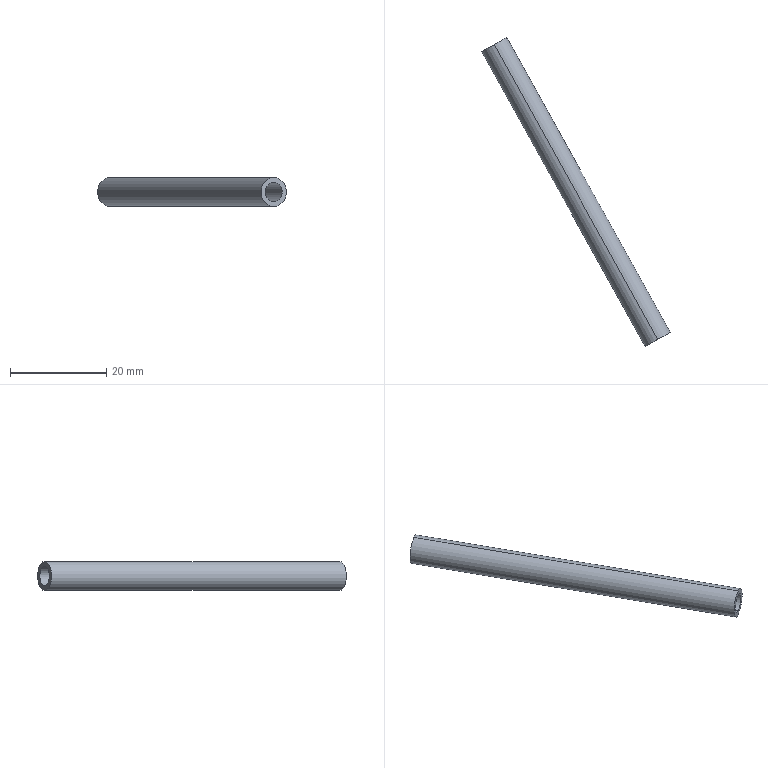Part | SolidWorks | features BaseBody 1 | 1 solid | 6 faces | box 39.184 x 64.132 x 6 mm | volume 1100 mm3 | cylinder 4 | plane 2 | commonest cylinder face diameters 4 x2 6 x2
STEP:
#1=CARTESIAN_POINT('',(-3.917,-65.903,-235.5));
#2=VERTEX_POINT('',#1);
#3=CARTESIAN_POINT('',(-3.917,-65.903,-231.5));
#4=VERTEX_POINT('',#3);
#5=CARTESIAN_POINT('',(-3.917,-65.903,-233.5));
#6=DIRECTION('',(0.4848,-0.8746,0.));
#7=DIRECTION('',(0.8746,0.4848,0.));
#8=AXIS2_PLACEMENT_3D('',#5,#6,#7);
#9=CIRCLE('',#8,2.);
#10=EDGE_CURVE('',#2,#4,#9,.T.);
#11=ORIENTED_EDGE('',*,*,#10,.T.);
#12=CARTESIAN_POINT('',(-37.854,-4.68,-231.5));
#13=VERTEX_POINT('',#12);
#14=CARTESIAN_POINT('',(-37.854,-4.68,-231.5));
#15=DIRECTION('',(-0.4848,0.8746,0.));
#16=VECTOR('',#15,1000.);
#17=LINE('',#14,#16);
#18=EDGE_CURVE('',#4,#13,#17,.T.);
#19=ORIENTED_EDGE('',*,*,#18,.T.);
#20=CARTESIAN_POINT('',(-37.854,-4.68,-235.5));
#21=VERTEX_POINT('',#20);
#22=CARTESIAN_POINT('',(-37.854,-4.68,-233.5));
#23=DIRECTION('',(0.4848,-0.8746,0.));
#24=DIRECTION('',(0.,0.,-1.));
#25=AXIS2_PLACEMENT_3D('',#22,#23,#24);
#26=CIRCLE('',#25,2.);
#27=EDGE_CURVE('',#21,#13,#26,.T.);
#28=ORIENTED_EDGE('',*,*,#27,.F.);
#29=CARTESIAN_POINT('',(-37.854,-4.68,-235.5));
#30=DIRECTION('',(-0.4848,0.8746,0.));
#31=VECTOR('',#30,1000.);
#32=LINE('',#29,#31);
#33=EDGE_CURVE('',#2,#21,#32,.T.);
#34=ORIENTED_EDGE('',*,*,#33,.F.);
#35=EDGE_LOOP('',(#11,#19,#28,#34));
#36=FACE_OUTER_BOUND('',#35,.T.);
#37=CARTESIAN_POINT('',(-37.854,-4.68,-233.5));
#38=DIRECTION('',(-0.4848,0.8746,0.));
#39=DIRECTION('',(0.,0.,-1.));
#40=AXIS2_PLACEMENT_3D('',#37,#38,#39);
#41=CYLINDRICAL_SURFACE('',#40,2.);
#42=ADVANCED_FACE('',(#36),#41,.F.);
#43=CARTESIAN_POINT('',(-3.917,-65.903,-230.5));
#44=VERTEX_POINT('',#43);
#45=CARTESIAN_POINT('',(-3.917,-65.903,-236.5));
#46=VERTEX_POINT('',#45);
#47=CARTESIAN_POINT('',(-3.917,-65.903,-233.5));
#48=DIRECTION('',(0.4848,-0.8746,0.));
#49=DIRECTION('',(0.8746,0.4848,0.));
#50=AXIS2_PLACEMENT_3D('',#47,#48,#49);
#51=CIRCLE('',#50,3.);
#52=EDGE_CURVE('',#44,#46,#51,.T.);
#53=ORIENTED_EDGE('',*,*,#52,.F.);
#54=CARTESIAN_POINT('',(-37.854,-4.68,-230.5));
#55=VERTEX_POINT('',#54);
#56=CARTESIAN_POINT('',(-37.854,-4.68,-230.5));
#57=DIRECTION('',(-0.4848,0.8746,0.));
#58=VECTOR('',#57,1000.);
#59=LINE('',#56,#58);
#60=EDGE_CURVE('',#44,#55,#59,.T.);
#61=ORIENTED_EDGE('',*,*,#60,.T.);
#62=CARTESIAN_POINT('',(-37.854,-4.68,-236.5));
#63=VERTEX_POINT('',#62);
#64=CARTESIAN_POINT('',(-37.854,-4.68,-233.5));
#65=DIRECTION('',(0.4848,-0.8746,0.));
#66=DIRECTION('',(0.,0.,-1.));
#67=AXIS2_PLACEMENT_3D('',#64,#65,#66);
#68=CIRCLE('',#67,3.);
#69=EDGE_CURVE('',#55,#63,#68,.T.);
#70=ORIENTED_EDGE('',*,*,#69,.T.);
#71=CARTESIAN_POINT('',(-37.854,-4.68,-236.5));
#72=DIRECTION('',(-0.4848,0.8746,0.));
#73=VECTOR('',#72,1000.);
#74=LINE('',#71,#73);
#75=EDGE_CURVE('',#46,#63,#74,.T.);
#76=ORIENTED_EDGE('',*,*,#75,.F.);
#77=EDGE_LOOP('',(#53,#61,#70,#76));
#78=FACE_OUTER_BOUND('',#77,.T.);
#79=CARTESIAN_POINT('',(-37.854,-4.68,-233.5));
#80=DIRECTION('',(-0.4848,0.8746,0.));
#81=DIRECTION('',(0.,0.,-1.));
#82=AXIS2_PLACEMENT_3D('',#79,#80,#81);
#83=CYLINDRICAL_SURFACE('',#82,3.);
#84=ADVANCED_FACE('',(#78),#83,.T.);
#85=ORIENTED_EDGE('',*,*,#60,.F.);
#86=CARTESIAN_POINT('',(-3.917,-65.903,-233.5));
#87=DIRECTION('',(0.4848,-0.8746,0.));
#88=DIRECTION('',(0.8746,0.4848,0.));
#89=AXIS2_PLACEMENT_3D('',#86,#87,#88);
#90=CIRCLE('',#89,3.);
#91=EDGE_CURVE('',#46,#44,#90,.T.);
#92=ORIENTED_EDGE('',*,*,#91,.F.);
#93=ORIENTED_EDGE('',*,*,#75,.T.);
#94=CARTESIAN_POINT('',(-37.854,-4.68,-233.5));
#95=DIRECTION('',(0.4848,-0.8746,0.));
#96=DIRECTION('',(0.,0.,-1.));
#97=AXIS2_PLACEMENT_3D('',#94,#95,#96);
#98=CIRCLE('',#97,3.);
#99=EDGE_CURVE('',#63,#55,#98,.T.);
#100=ORIENTED_EDGE('',*,*,#99,.T.);
#101=EDGE_LOOP('',(#85,#92,#93,#100));
#102=FACE_OUTER_BOUND('',#101,.T.);
#103=CARTESIAN_POINT('',(-37.854,-4.68,-233.5));
#104=DIRECTION('',(-0.4848,0.8746,0.));
#105=DIRECTION('',(0.,0.,-1.));
#106=AXIS2_PLACEMENT_3D('',#103,#104,#105);
#107=CYLINDRICAL_SURFACE('',#106,3.);
#108=ADVANCED_FACE('',(#102),#107,.T.);
#109=ORIENTED_EDGE('',*,*,#10,.F.);
#110=CARTESIAN_POINT('',(-3.917,-65.903,-233.5));
#111=DIRECTION('',(0.4848,-0.8746,0.));
#112=DIRECTION('',(0.8746,0.4848,0.));
#113=AXIS2_PLACEMENT_3D('',#110,#111,#112);
#114=CIRCLE('',#113,2.);
#115=EDGE_CURVE('',#4,#2,#114,.T.);
#116=ORIENTED_EDGE('',*,*,#115,.F.);
#117=EDGE_LOOP('',(#109,#116));
#118=FACE_BOUND('',#117,.T.);
#119=ORIENTED_EDGE('',*,*,#91,.T.);
#120=ORIENTED_EDGE('',*,*,#52,.T.);
#121=EDGE_LOOP('',(#119,#120));
#122=FACE_OUTER_BOUND('',#121,.T.);
#123=CARTESIAN_POINT('',(-1.293,-64.449,-233.5));
#124=DIRECTION('',(0.4848,-0.8746,0.));
#125=DIRECTION('',(0.,0.,1.));
#126=AXIS2_PLACEMENT_3D('',#123,#124,#125);
#127=PLANE('',#126);
#128=ADVANCED_FACE('',(#118,#122),#127,.T.);
#129=ORIENTED_EDGE('',*,*,#18,.F.);
#130=ORIENTED_EDGE('',*,*,#115,.T.);
#131=ORIENTED_EDGE('',*,*,#33,.T.);
#132=CARTESIAN_POINT('',(-37.854,-4.68,-233.5));
#133=DIRECTION('',(0.4848,-0.8746,0.));
#134=DIRECTION('',(0.,0.,-1.));
#135=AXIS2_PLACEMENT_3D('',#132,#133,#134);
#136=CIRCLE('',#135,2.);
#137=EDGE_CURVE('',#13,#21,#136,.T.);
#138=ORIENTED_EDGE('',*,*,#137,.F.);
#139=EDGE_LOOP('',(#129,#130,#131,#138));
#140=FACE_OUTER_BOUND('',#139,.T.);
#141=CARTESIAN_POINT('',(-37.854,-4.68,-233.5));
#142=DIRECTION('',(-0.4848,0.8746,0.));
#143=DIRECTION('',(0.,0.,-1.));
#144=AXIS2_PLACEMENT_3D('',#141,#142,#143);
#145=CYLINDRICAL_SURFACE('',#144,2.);
#146=ADVANCED_FACE('',(#140),#145,.F.);
#147=ORIENTED_EDGE('',*,*,#99,.F.);
#148=ORIENTED_EDGE('',*,*,#69,.F.);
#149=EDGE_LOOP('',(#147,#148));
#150=FACE_OUTER_BOUND('',#149,.T.);
#151=ORIENTED_EDGE('',*,*,#27,.T.);
#152=ORIENTED_EDGE('',*,*,#137,.T.);
#153=EDGE_LOOP('',(#151,#152));
#154=FACE_BOUND('',#153,.T.);
#155=CARTESIAN_POINT('',(-36.104,-3.711,-233.5));
#156=DIRECTION('',(-0.4848,0.8746,0.));
#157=DIRECTION('',(0.,0.,-1.));
#158=AXIS2_PLACEMENT_3D('',#155,#156,#157);
#159=PLANE('',#158);
#160=ADVANCED_FACE('',(#150,#154),#159,.T.);
#161=CLOSED_SHELL('',(#42,#84,#108,#128,#146,#160));
#162=MANIFOLD_SOLID_BREP('',#161);
#163=CARTESIAN_POINT('',(0.,0.,0.));
#164=DIRECTION('',(0.,0.,1.));
#165=DIRECTION('',(1.,0.,0.));
#166=AXIS2_PLACEMENT_3D('',#163,#164,#165);
#167=(LENGTH_UNIT()NAMED_UNIT(*)SI_UNIT(.MILLI.,.METRE.));
#168=UNCERTAINTY_MEASURE_WITH_UNIT(LENGTH_MEASURE(0.00001),#167,'','');
#169=(NAMED_UNIT(*)PLANE_ANGLE_UNIT()SI_UNIT($,.RADIAN.));
#170=(NAMED_UNIT(*)SI_UNIT($,.STERADIAN.)SOLID_ANGLE_UNIT());
#171=(GEOMETRIC_REPRESENTATION_CONTEXT(3)GLOBAL_UNCERTAINTY_ASSIGNED_CONTEXT((#168))GLOBAL_UNIT_ASSIGNED_CONTEXT((#167,#169,#170))REPRESENTATION_CONTEXT('',''));
#172=ADVANCED_BREP_SHAPE_REPRESENTATION('',(#162,#166),#171);